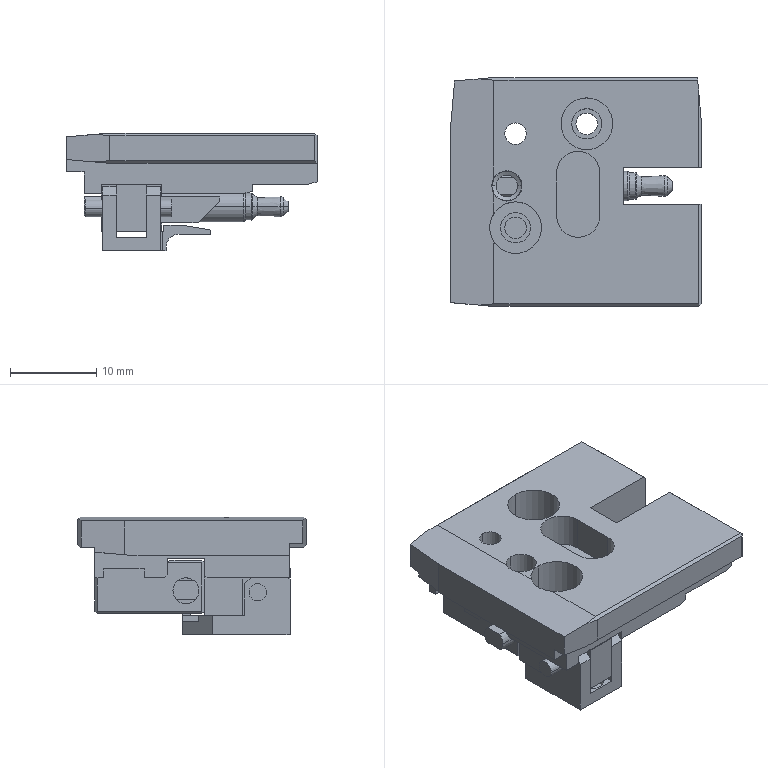Part | NX | 7 solids | 233 faces | box 29 x 26.5 x 13.65 mm | volume 4617 mm3 | plane 165 | cylinder 50 | cone 10 | torus 8 | commonest cylinder face diameters 2 x8 2.5 x8 3.5 x8 3.1 x6 6 x6 3 x5